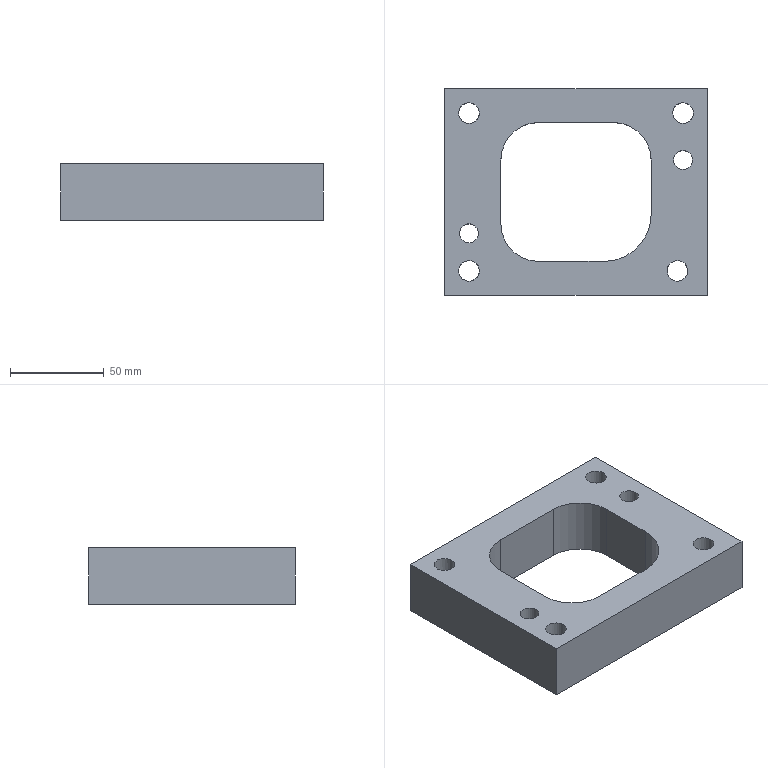Part | STEP file | 200_id686_x_t | 1 solid | 32 faces | box 140 x 110 x 30 mm | volume 271786 mm3 | plane 16 | cylinder 16 | commonest cylinder face diameters 11 x6 17 x4 40 x3 10 x2 50 x1